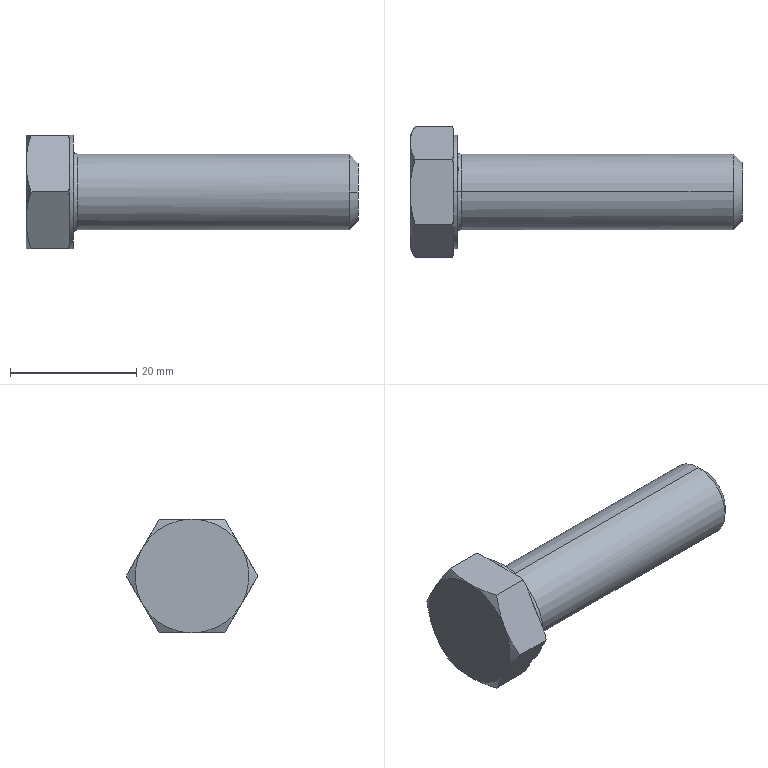Part | STEP file | 1 solid | 35 faces | box 52.5 x 20.785 x 18 mm | volume 7141 mm3 | plane 15 | cone 14 | cylinder 4 | spline 2 | commonest cylinder face diameters 12 x2 18 x2